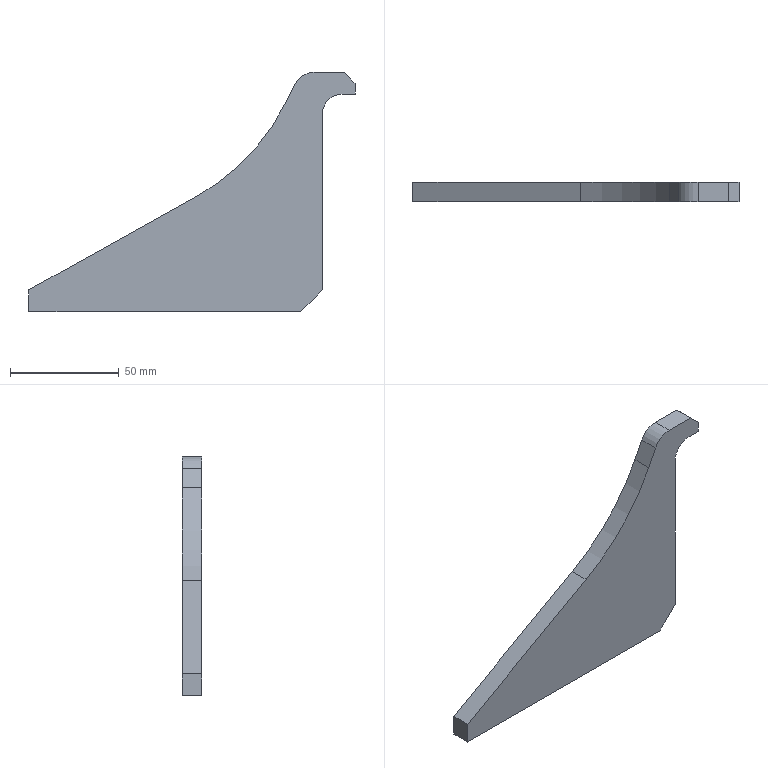Part | SolidWorks | features FlatPattern 1, SMBaseFlange 1, SheetMetal 1 | 1 solid | 15 faces | box 150 x 9 x 110 mm | volume 64944 mm3 | plane 12 | cylinder 3 | commonest cylinder face diameters 18 x1 20 x1 200 x1
STEP:
#1=CARTESIAN_POINT('',(0.,0.,0.));
#2=VERTEX_POINT('',#1);
#3=CARTESIAN_POINT('',(0.,0.,10.));
#4=VERTEX_POINT('',#3);
#5=CARTESIAN_POINT('',(0.,0.,10.));
#6=DIRECTION('',(0.,0.,1.));
#7=VECTOR('',#6,1000.);
#8=LINE('',#5,#7);
#9=EDGE_CURVE('',#2,#4,#8,.T.);
#10=ORIENTED_EDGE('',*,*,#9,.F.);
#11=CARTESIAN_POINT('',(0.,-9.,0.));
#12=VERTEX_POINT('',#11);
#13=CARTESIAN_POINT('',(0.,-9.,0.));
#14=DIRECTION('',(0.,1.,0.));
#15=VECTOR('',#14,1000.);
#16=LINE('',#13,#15);
#17=EDGE_CURVE('',#12,#2,#16,.T.);
#18=ORIENTED_EDGE('',*,*,#17,.F.);
#19=CARTESIAN_POINT('',(0.,-9.,10.));
#20=VERTEX_POINT('',#19);
#21=CARTESIAN_POINT('',(0.,-9.,10.));
#22=DIRECTION('',(0.,0.,1.));
#23=VECTOR('',#22,1000.);
#24=LINE('',#21,#23);
#25=EDGE_CURVE('',#12,#20,#24,.T.);
#26=ORIENTED_EDGE('',*,*,#25,.T.);
#27=CARTESIAN_POINT('',(0.,-9.,10.));
#28=DIRECTION('',(0.,1.,0.));
#29=VECTOR('',#28,1000.);
#30=LINE('',#27,#29);
#31=EDGE_CURVE('',#20,#4,#30,.T.);
#32=ORIENTED_EDGE('',*,*,#31,.T.);
#33=EDGE_LOOP('',(#10,#18,#26,#32));
#34=FACE_OUTER_BOUND('',#33,.T.);
#35=CARTESIAN_POINT('',(0.,-9.,10.));
#36=DIRECTION('',(-1.,0.,0.));
#37=DIRECTION('',(0.,0.,1.));
#38=AXIS2_PLACEMENT_3D('',#35,#36,#37);
#39=PLANE('',#38);
#40=ADVANCED_FACE('',(#34),#39,.T.);
#41=CARTESIAN_POINT('',(125.,0.,0.));
#42=VERTEX_POINT('',#41);
#43=CARTESIAN_POINT('',(0.,0.,0.));
#44=DIRECTION('',(-1.,0.,0.));
#45=VECTOR('',#44,1000.);
#46=LINE('',#43,#45);
#47=EDGE_CURVE('',#42,#2,#46,.T.);
#48=ORIENTED_EDGE('',*,*,#47,.F.);
#49=CARTESIAN_POINT('',(125.,-9.,0.));
#50=VERTEX_POINT('',#49);
#51=CARTESIAN_POINT('',(125.,-9.,0.));
#52=DIRECTION('',(0.,1.,0.));
#53=VECTOR('',#52,1000.);
#54=LINE('',#51,#53);
#55=EDGE_CURVE('',#50,#42,#54,.T.);
#56=ORIENTED_EDGE('',*,*,#55,.F.);
#57=CARTESIAN_POINT('',(0.,-9.,0.));
#58=DIRECTION('',(-1.,0.,0.));
#59=VECTOR('',#58,1000.);
#60=LINE('',#57,#59);
#61=EDGE_CURVE('',#50,#12,#60,.T.);
#62=ORIENTED_EDGE('',*,*,#61,.T.);
#63=ORIENTED_EDGE('',*,*,#17,.T.);
#64=EDGE_LOOP('',(#48,#56,#62,#63));
#65=FACE_OUTER_BOUND('',#64,.T.);
#66=CARTESIAN_POINT('',(0.,-9.,0.));
#67=DIRECTION('',(0.,0.,-1.));
#68=DIRECTION('',(-1.,0.,0.));
#69=AXIS2_PLACEMENT_3D('',#66,#67,#68);
#70=PLANE('',#69);
#71=ADVANCED_FACE('',(#65),#70,.T.);
#72=CARTESIAN_POINT('',(135.,0.,10.));
#73=VERTEX_POINT('',#72);
#74=CARTESIAN_POINT('',(125.,0.,0.));
#75=DIRECTION('',(-0.7071,0.,-0.7071));
#76=VECTOR('',#75,1000.);
#77=LINE('',#74,#76);
#78=EDGE_CURVE('',#73,#42,#77,.T.);
#79=ORIENTED_EDGE('',*,*,#78,.F.);
#80=CARTESIAN_POINT('',(135.,-9.,10.));
#81=VERTEX_POINT('',#80);
#82=CARTESIAN_POINT('',(135.,-9.,10.));
#83=DIRECTION('',(0.,1.,0.));
#84=VECTOR('',#83,1000.);
#85=LINE('',#82,#84);
#86=EDGE_CURVE('',#81,#73,#85,.T.);
#87=ORIENTED_EDGE('',*,*,#86,.F.);
#88=CARTESIAN_POINT('',(125.,-9.,0.));
#89=DIRECTION('',(-0.7071,0.,-0.7071));
#90=VECTOR('',#89,1000.);
#91=LINE('',#88,#90);
#92=EDGE_CURVE('',#81,#50,#91,.T.);
#93=ORIENTED_EDGE('',*,*,#92,.T.);
#94=ORIENTED_EDGE('',*,*,#55,.T.);
#95=EDGE_LOOP('',(#79,#87,#93,#94));
#96=FACE_OUTER_BOUND('',#95,.T.);
#97=CARTESIAN_POINT('',(125.,-9.,0.));
#98=DIRECTION('',(0.7071,0.,-0.7071));
#99=DIRECTION('',(-0.7071,0.,-0.7071));
#100=AXIS2_PLACEMENT_3D('',#97,#98,#99);
#101=PLANE('',#100);
#102=ADVANCED_FACE('',(#96),#101,.T.);
#103=CARTESIAN_POINT('',(135.,0.,91.));
#104=VERTEX_POINT('',#103);
#105=CARTESIAN_POINT('',(135.,0.,10.));
#106=DIRECTION('',(0.,0.,-1.));
#107=VECTOR('',#106,1000.);
#108=LINE('',#105,#107);
#109=EDGE_CURVE('',#104,#73,#108,.T.);
#110=ORIENTED_EDGE('',*,*,#109,.F.);
#111=CARTESIAN_POINT('',(135.,-9.,91.));
#112=VERTEX_POINT('',#111);
#113=CARTESIAN_POINT('',(135.,-9.,91.));
#114=DIRECTION('',(0.,1.,0.));
#115=VECTOR('',#114,1000.);
#116=LINE('',#113,#115);
#117=EDGE_CURVE('',#112,#104,#116,.T.);
#118=ORIENTED_EDGE('',*,*,#117,.F.);
#119=CARTESIAN_POINT('',(135.,-9.,10.));
#120=DIRECTION('',(0.,0.,-1.));
#121=VECTOR('',#120,1000.);
#122=LINE('',#119,#121);
#123=EDGE_CURVE('',#112,#81,#122,.T.);
#124=ORIENTED_EDGE('',*,*,#123,.T.);
#125=ORIENTED_EDGE('',*,*,#86,.T.);
#126=EDGE_LOOP('',(#110,#118,#124,#125));
#127=FACE_OUTER_BOUND('',#126,.T.);
#128=CARTESIAN_POINT('',(135.,-9.,10.));
#129=DIRECTION('',(1.,0.,0.));
#130=DIRECTION('',(0.,0.,-1.));
#131=AXIS2_PLACEMENT_3D('',#128,#129,#130);
#132=PLANE('',#131);
#133=ADVANCED_FACE('',(#127),#132,.T.);
#134=CARTESIAN_POINT('',(144.,0.,100.));
#135=VERTEX_POINT('',#134);
#136=CARTESIAN_POINT('',(144.,0.,91.));
#137=DIRECTION('',(0.,-1.,0.));
#138=DIRECTION('',(0.,0.,-1.));
#139=AXIS2_PLACEMENT_3D('',#136,#137,#138);
#140=CIRCLE('',#139,9.);
#141=EDGE_CURVE('',#135,#104,#140,.T.);
#142=ORIENTED_EDGE('',*,*,#141,.F.);
#143=CARTESIAN_POINT('',(144.,-9.,100.));
#144=VERTEX_POINT('',#143);
#145=CARTESIAN_POINT('',(144.,-9.,100.));
#146=DIRECTION('',(0.,1.,0.));
#147=VECTOR('',#146,1000.);
#148=LINE('',#145,#147);
#149=EDGE_CURVE('',#144,#135,#148,.T.);
#150=ORIENTED_EDGE('',*,*,#149,.F.);
#151=CARTESIAN_POINT('',(144.,-9.,91.));
#152=DIRECTION('',(0.,-1.,0.));
#153=DIRECTION('',(0.,0.,-1.));
#154=AXIS2_PLACEMENT_3D('',#151,#152,#153);
#155=CIRCLE('',#154,9.);
#156=EDGE_CURVE('',#144,#112,#155,.T.);
#157=ORIENTED_EDGE('',*,*,#156,.T.);
#158=ORIENTED_EDGE('',*,*,#117,.T.);
#159=EDGE_LOOP('',(#142,#150,#157,#158));
#160=FACE_OUTER_BOUND('',#159,.T.);
#161=CARTESIAN_POINT('',(144.,-9.,91.));
#162=DIRECTION('',(0.,1.,0.));
#163=DIRECTION('',(0.,0.,1.));
#164=AXIS2_PLACEMENT_3D('',#161,#162,#163);
#165=CYLINDRICAL_SURFACE('',#164,9.);
#166=ADVANCED_FACE('',(#160),#165,.F.);
#167=CARTESIAN_POINT('',(150.,0.,100.));
#168=VERTEX_POINT('',#167);
#169=CARTESIAN_POINT('',(144.,0.,100.));
#170=DIRECTION('',(-1.,0.,0.));
#171=VECTOR('',#170,1000.);
#172=LINE('',#169,#171);
#173=EDGE_CURVE('',#168,#135,#172,.T.);
#174=ORIENTED_EDGE('',*,*,#173,.F.);
#175=CARTESIAN_POINT('',(150.,-9.,100.));
#176=VERTEX_POINT('',#175);
#177=CARTESIAN_POINT('',(150.,-9.,100.));
#178=DIRECTION('',(0.,1.,0.));
#179=VECTOR('',#178,1000.);
#180=LINE('',#177,#179);
#181=EDGE_CURVE('',#176,#168,#180,.T.);
#182=ORIENTED_EDGE('',*,*,#181,.F.);
#183=CARTESIAN_POINT('',(144.,-9.,100.));
#184=DIRECTION('',(-1.,0.,0.));
#185=VECTOR('',#184,1000.);
#186=LINE('',#183,#185);
#187=EDGE_CURVE('',#176,#144,#186,.T.);
#188=ORIENTED_EDGE('',*,*,#187,.T.);
#189=ORIENTED_EDGE('',*,*,#149,.T.);
#190=EDGE_LOOP('',(#174,#182,#188,#189));
#191=FACE_OUTER_BOUND('',#190,.T.);
#192=CARTESIAN_POINT('',(144.,-9.,100.));
#193=DIRECTION('',(0.,0.,-1.));
#194=DIRECTION('',(-1.,0.,0.));
#195=AXIS2_PLACEMENT_3D('',#192,#193,#194);
#196=PLANE('',#195);
#197=ADVANCED_FACE('',(#191),#196,.T.);
#198=CARTESIAN_POINT('',(150.,0.,105.));
#199=VERTEX_POINT('',#198);
#200=CARTESIAN_POINT('',(150.,0.,100.));
#201=DIRECTION('',(0.,0.,-1.));
#202=VECTOR('',#201,1000.);
#203=LINE('',#200,#202);
#204=EDGE_CURVE('',#199,#168,#203,.T.);
#205=ORIENTED_EDGE('',*,*,#204,.F.);
#206=CARTESIAN_POINT('',(150.,-9.,105.));
#207=VERTEX_POINT('',#206);
#208=CARTESIAN_POINT('',(150.,-9.,105.));
#209=DIRECTION('',(0.,1.,0.));
#210=VECTOR('',#209,1000.);
#211=LINE('',#208,#210);
#212=EDGE_CURVE('',#207,#199,#211,.T.);
#213=ORIENTED_EDGE('',*,*,#212,.F.);
#214=CARTESIAN_POINT('',(150.,-9.,100.));
#215=DIRECTION('',(0.,0.,-1.));
#216=VECTOR('',#215,1000.);
#217=LINE('',#214,#216);
#218=EDGE_CURVE('',#207,#176,#217,.T.);
#219=ORIENTED_EDGE('',*,*,#218,.T.);
#220=ORIENTED_EDGE('',*,*,#181,.T.);
#221=EDGE_LOOP('',(#205,#213,#219,#220));
#222=FACE_OUTER_BOUND('',#221,.T.);
#223=CARTESIAN_POINT('',(150.,-9.,100.));
#224=DIRECTION('',(1.,0.,0.));
#225=DIRECTION('',(0.,0.,-1.));
#226=AXIS2_PLACEMENT_3D('',#223,#224,#225);
#227=PLANE('',#226);
#228=ADVANCED_FACE('',(#222),#227,.T.);
#229=CARTESIAN_POINT('',(145.,0.,110.));
#230=VERTEX_POINT('',#229);
#231=CARTESIAN_POINT('',(150.,0.,105.));
#232=DIRECTION('',(0.7071,0.,-0.7071));
#233=VECTOR('',#232,1000.);
#234=LINE('',#231,#233);
#235=EDGE_CURVE('',#230,#199,#234,.T.);
#236=ORIENTED_EDGE('',*,*,#235,.F.);
#237=CARTESIAN_POINT('',(145.,-9.,110.));
#238=VERTEX_POINT('',#237);
#239=CARTESIAN_POINT('',(145.,-9.,110.));
#240=DIRECTION('',(0.,1.,0.));
#241=VECTOR('',#240,1000.);
#242=LINE('',#239,#241);
#243=EDGE_CURVE('',#238,#230,#242,.T.);
#244=ORIENTED_EDGE('',*,*,#243,.F.);
#245=CARTESIAN_POINT('',(150.,-9.,105.));
#246=DIRECTION('',(0.7071,0.,-0.7071));
#247=VECTOR('',#246,1000.);
#248=LINE('',#245,#247);
#249=EDGE_CURVE('',#238,#207,#248,.T.);
#250=ORIENTED_EDGE('',*,*,#249,.T.);
#251=ORIENTED_EDGE('',*,*,#212,.T.);
#252=EDGE_LOOP('',(#236,#244,#250,#251));
#253=FACE_OUTER_BOUND('',#252,.T.);
#254=CARTESIAN_POINT('',(150.,-9.,105.));
#255=DIRECTION('',(0.7071,0.,0.7071));
#256=DIRECTION('',(0.7071,0.,-0.7071));
#257=AXIS2_PLACEMENT_3D('',#254,#255,#256);
#258=PLANE('',#257);
#259=ADVANCED_FACE('',(#253),#258,.T.);
#260=CARTESIAN_POINT('',(131.18,0.,110.));
#261=VERTEX_POINT('',#260);
#262=CARTESIAN_POINT('',(145.,0.,110.));
#263=DIRECTION('',(1.,0.,0.));
#264=VECTOR('',#263,1000.);
#265=LINE('',#262,#264);
#266=EDGE_CURVE('',#261,#230,#265,.T.);
#267=ORIENTED_EDGE('',*,*,#266,.F.);
#268=CARTESIAN_POINT('',(131.18,-9.,110.));
#269=VERTEX_POINT('',#268);
#270=CARTESIAN_POINT('',(131.18,-9.,110.));
#271=DIRECTION('',(0.,1.,0.));
#272=VECTOR('',#271,1000.);
#273=LINE('',#270,#272);
#274=EDGE_CURVE('',#269,#261,#273,.T.);
#275=ORIENTED_EDGE('',*,*,#274,.F.);
#276=CARTESIAN_POINT('',(145.,-9.,110.));
#277=DIRECTION('',(1.,0.,0.));
#278=VECTOR('',#277,1000.);
#279=LINE('',#276,#278);
#280=EDGE_CURVE('',#269,#238,#279,.T.);
#281=ORIENTED_EDGE('',*,*,#280,.T.);
#282=ORIENTED_EDGE('',*,*,#243,.T.);
#283=EDGE_LOOP('',(#267,#275,#281,#282));
#284=FACE_OUTER_BOUND('',#283,.T.);
#285=CARTESIAN_POINT('',(145.,-9.,110.));
#286=DIRECTION('',(0.,0.,1.));
#287=DIRECTION('',(1.,0.,0.));
#288=AXIS2_PLACEMENT_3D('',#285,#286,#287);
#289=PLANE('',#288);
#290=ADVANCED_FACE('',(#284),#289,.T.);
#291=CARTESIAN_POINT('',(122.236,0.,104.472));
#292=VERTEX_POINT('',#291);
#293=CARTESIAN_POINT('',(131.18,0.,100.));
#294=DIRECTION('',(0.,1.,0.));
#295=DIRECTION('',(0.,0.,-1.));
#296=AXIS2_PLACEMENT_3D('',#293,#294,#295);
#297=CIRCLE('',#296,10.);
#298=EDGE_CURVE('',#292,#261,#297,.T.);
#299=ORIENTED_EDGE('',*,*,#298,.F.);
#300=CARTESIAN_POINT('',(122.236,-9.,104.472));
#301=VERTEX_POINT('',#300);
#302=CARTESIAN_POINT('',(122.236,-9.,104.472));
#303=DIRECTION('',(0.,1.,0.));
#304=VECTOR('',#303,1000.);
#305=LINE('',#302,#304);
#306=EDGE_CURVE('',#301,#292,#305,.T.);
#307=ORIENTED_EDGE('',*,*,#306,.F.);
#308=CARTESIAN_POINT('',(131.18,-9.,100.));
#309=DIRECTION('',(0.,1.,0.));
#310=DIRECTION('',(0.,0.,-1.));
#311=AXIS2_PLACEMENT_3D('',#308,#309,#310);
#312=CIRCLE('',#311,10.);
#313=EDGE_CURVE('',#301,#269,#312,.T.);
#314=ORIENTED_EDGE('',*,*,#313,.T.);
#315=ORIENTED_EDGE('',*,*,#274,.T.);
#316=EDGE_LOOP('',(#299,#307,#314,#315));
#317=FACE_OUTER_BOUND('',#316,.T.);
#318=CARTESIAN_POINT('',(131.18,-9.,100.));
#319=DIRECTION('',(0.,1.,0.));
#320=DIRECTION('',(0.,0.,1.));
#321=AXIS2_PLACEMENT_3D('',#318,#319,#320);
#322=CYLINDRICAL_SURFACE('',#321,10.);
#323=ADVANCED_FACE('',(#317),#322,.T.);
#324=CARTESIAN_POINT('',(117.795,0.,95.59));
#325=VERTEX_POINT('',#324);
#326=CARTESIAN_POINT('',(122.236,0.,104.472));
#327=DIRECTION('',(0.4472,0.,0.8944));
#328=VECTOR('',#327,1000.);
#329=LINE('',#326,#328);
#330=EDGE_CURVE('',#325,#292,#329,.T.);
#331=ORIENTED_EDGE('',*,*,#330,.F.);
#332=CARTESIAN_POINT('',(117.795,-9.,95.59));
#333=VERTEX_POINT('',#332);
#334=CARTESIAN_POINT('',(117.795,-9.,95.59));
#335=DIRECTION('',(0.,1.,0.));
#336=VECTOR('',#335,1000.);
#337=LINE('',#334,#336);
#338=EDGE_CURVE('',#333,#325,#337,.T.);
#339=ORIENTED_EDGE('',*,*,#338,.F.);
#340=CARTESIAN_POINT('',(122.236,-9.,104.472));
#341=DIRECTION('',(0.4472,0.,0.8944));
#342=VECTOR('',#341,1000.);
#343=LINE('',#340,#342);
#344=EDGE_CURVE('',#333,#301,#343,.T.);
#345=ORIENTED_EDGE('',*,*,#344,.T.);
#346=ORIENTED_EDGE('',*,*,#306,.T.);
#347=EDGE_LOOP('',(#331,#339,#345,#346));
#348=FACE_OUTER_BOUND('',#347,.T.);
#349=CARTESIAN_POINT('',(122.236,-9.,104.472));
#350=DIRECTION('',(-0.8944,0.,0.4472));
#351=DIRECTION('',(0.4472,0.,0.8944));
#352=AXIS2_PLACEMENT_3D('',#349,#350,#351);
#353=PLANE('',#352);
#354=ADVANCED_FACE('',(#348),#353,.T.);
#355=CARTESIAN_POINT('',(77.059,0.,52.975));
#356=VERTEX_POINT('',#355);
#357=CARTESIAN_POINT('',(28.352,0.,140.312));
#358=DIRECTION('',(0.,-1.,0.));
#359=DIRECTION('',(0.,0.,1.));
#360=AXIS2_PLACEMENT_3D('',#357,#358,#359);
#361=CIRCLE('',#360,100.);
#362=EDGE_CURVE('',#356,#325,#361,.T.);
#363=ORIENTED_EDGE('',*,*,#362,.F.);
#364=CARTESIAN_POINT('',(77.059,-9.,52.975));
#365=VERTEX_POINT('',#364);
#366=CARTESIAN_POINT('',(77.059,-9.,52.975));
#367=DIRECTION('',(0.,1.,0.));
#368=VECTOR('',#367,1000.);
#369=LINE('',#366,#368);
#370=EDGE_CURVE('',#365,#356,#369,.T.);
#371=ORIENTED_EDGE('',*,*,#370,.F.);
#372=CARTESIAN_POINT('',(28.352,-9.,140.312));
#373=DIRECTION('',(0.,-1.,0.));
#374=DIRECTION('',(0.,0.,1.));
#375=AXIS2_PLACEMENT_3D('',#372,#373,#374);
#376=CIRCLE('',#375,100.);
#377=EDGE_CURVE('',#365,#333,#376,.T.);
#378=ORIENTED_EDGE('',*,*,#377,.T.);
#379=ORIENTED_EDGE('',*,*,#338,.T.);
#380=EDGE_LOOP('',(#363,#371,#378,#379));
#381=FACE_OUTER_BOUND('',#380,.T.);
#382=CARTESIAN_POINT('',(28.352,-9.,140.312));
#383=DIRECTION('',(0.,1.,0.));
#384=DIRECTION('',(0.,0.,1.));
#385=AXIS2_PLACEMENT_3D('',#382,#383,#384);
#386=CYLINDRICAL_SURFACE('',#385,100.);
#387=ADVANCED_FACE('',(#381),#386,.F.);
#388=CARTESIAN_POINT('',(77.059,0.,52.975));
#389=DIRECTION('',(0.8734,0.,0.4871));
#390=VECTOR('',#389,1000.);
#391=LINE('',#388,#390);
#392=EDGE_CURVE('',#4,#356,#391,.T.);
#393=ORIENTED_EDGE('',*,*,#392,.F.);
#394=ORIENTED_EDGE('',*,*,#31,.F.);
#395=CARTESIAN_POINT('',(77.059,-9.,52.975));
#396=DIRECTION('',(0.8734,0.,0.4871));
#397=VECTOR('',#396,1000.);
#398=LINE('',#395,#397);
#399=EDGE_CURVE('',#20,#365,#398,.T.);
#400=ORIENTED_EDGE('',*,*,#399,.T.);
#401=ORIENTED_EDGE('',*,*,#370,.T.);
#402=EDGE_LOOP('',(#393,#394,#400,#401));
#403=FACE_OUTER_BOUND('',#402,.T.);
#404=CARTESIAN_POINT('',(77.059,-9.,52.975));
#405=DIRECTION('',(-0.4871,0.,0.8734));
#406=DIRECTION('',(0.8734,0.,0.4871));
#407=AXIS2_PLACEMENT_3D('',#404,#405,#406);
#408=PLANE('',#407);
#409=ADVANCED_FACE('',(#403),#408,.T.);
#410=ORIENTED_EDGE('',*,*,#25,.F.);
#411=ORIENTED_EDGE('',*,*,#61,.F.);
#412=ORIENTED_EDGE('',*,*,#92,.F.);
#413=ORIENTED_EDGE('',*,*,#123,.F.);
#414=ORIENTED_EDGE('',*,*,#156,.F.);
#415=ORIENTED_EDGE('',*,*,#187,.F.);
#416=ORIENTED_EDGE('',*,*,#218,.F.);
#417=ORIENTED_EDGE('',*,*,#249,.F.);
#418=ORIENTED_EDGE('',*,*,#280,.F.);
#419=ORIENTED_EDGE('',*,*,#313,.F.);
#420=ORIENTED_EDGE('',*,*,#344,.F.);
#421=ORIENTED_EDGE('',*,*,#377,.F.);
#422=ORIENTED_EDGE('',*,*,#399,.F.);
#423=EDGE_LOOP('',(#410,#411,#412,#413,#414,#415,#416,#417,#418,#419,#420,#421,#422));
#424=FACE_OUTER_BOUND('',#423,.T.);
#425=CARTESIAN_POINT('',(144.,-9.,91.));
#426=DIRECTION('',(0.,-1.,0.));
#427=DIRECTION('',(0.,0.,-1.));
#428=AXIS2_PLACEMENT_3D('',#425,#426,#427);
#429=PLANE('',#428);
#430=ADVANCED_FACE('',(#424),#429,.T.);
#431=ORIENTED_EDGE('',*,*,#9,.T.);
#432=ORIENTED_EDGE('',*,*,#392,.T.);
#433=ORIENTED_EDGE('',*,*,#362,.T.);
#434=ORIENTED_EDGE('',*,*,#330,.T.);
#435=ORIENTED_EDGE('',*,*,#298,.T.);
#436=ORIENTED_EDGE('',*,*,#266,.T.);
#437=ORIENTED_EDGE('',*,*,#235,.T.);
#438=ORIENTED_EDGE('',*,*,#204,.T.);
#439=ORIENTED_EDGE('',*,*,#173,.T.);
#440=ORIENTED_EDGE('',*,*,#141,.T.);
#441=ORIENTED_EDGE('',*,*,#109,.T.);
#442=ORIENTED_EDGE('',*,*,#78,.T.);
#443=ORIENTED_EDGE('',*,*,#47,.T.);
#444=EDGE_LOOP('',(#431,#432,#433,#434,#435,#436,#437,#438,#439,#440,#441,#442,#443));
#445=FACE_OUTER_BOUND('',#444,.T.);
#446=CARTESIAN_POINT('',(144.,0.,91.));
#447=DIRECTION('',(0.,-1.,0.));
#448=DIRECTION('',(0.,0.,-1.));
#449=AXIS2_PLACEMENT_3D('',#446,#447,#448);
#450=PLANE('',#449);
#451=ADVANCED_FACE('',(#445),#450,.F.);
#452=CLOSED_SHELL('',(#40,#71,#102,#133,#166,#197,#228,#259,#290,#323,#354,#387,#409,#430,#451));
#453=MANIFOLD_SOLID_BREP('',#452);
#454=CARTESIAN_POINT('',(0.,0.,0.));
#455=DIRECTION('',(0.,0.,1.));
#456=DIRECTION('',(1.,0.,0.));
#457=AXIS2_PLACEMENT_3D('',#454,#455,#456);
#458=(LENGTH_UNIT()NAMED_UNIT(*)SI_UNIT(.MILLI.,.METRE.));
#459=UNCERTAINTY_MEASURE_WITH_UNIT(LENGTH_MEASURE(0.00001),#458,'','');
#460=(NAMED_UNIT(*)PLANE_ANGLE_UNIT()SI_UNIT($,.RADIAN.));
#461=(NAMED_UNIT(*)SI_UNIT($,.STERADIAN.)SOLID_ANGLE_UNIT());
#462=(GEOMETRIC_REPRESENTATION_CONTEXT(3)GLOBAL_UNCERTAINTY_ASSIGNED_CONTEXT((#459))GLOBAL_UNIT_ASSIGNED_CONTEXT((#458,#460,#461))REPRESENTATION_CONTEXT('',''));
#463=ADVANCED_BREP_SHAPE_REPRESENTATION('',(#453,#457),#462);